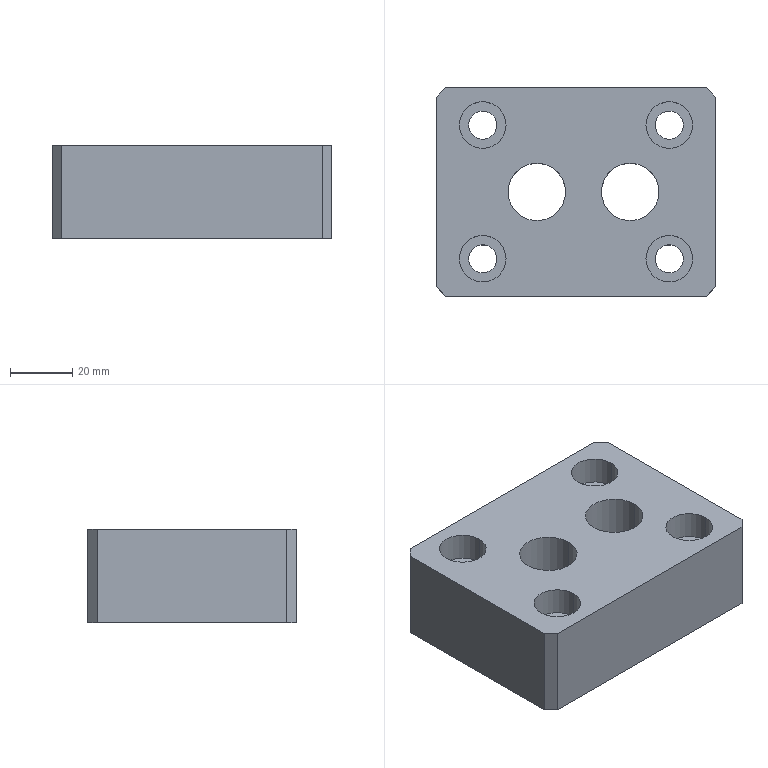Part | STEP file | 1 solid | 34 faces | box 90 x 67 x 30 mm | volume 152526 mm3 | cylinder 20 | plane 14 | commonest cylinder face diameters 9 x8 15 x8 18.5 x4